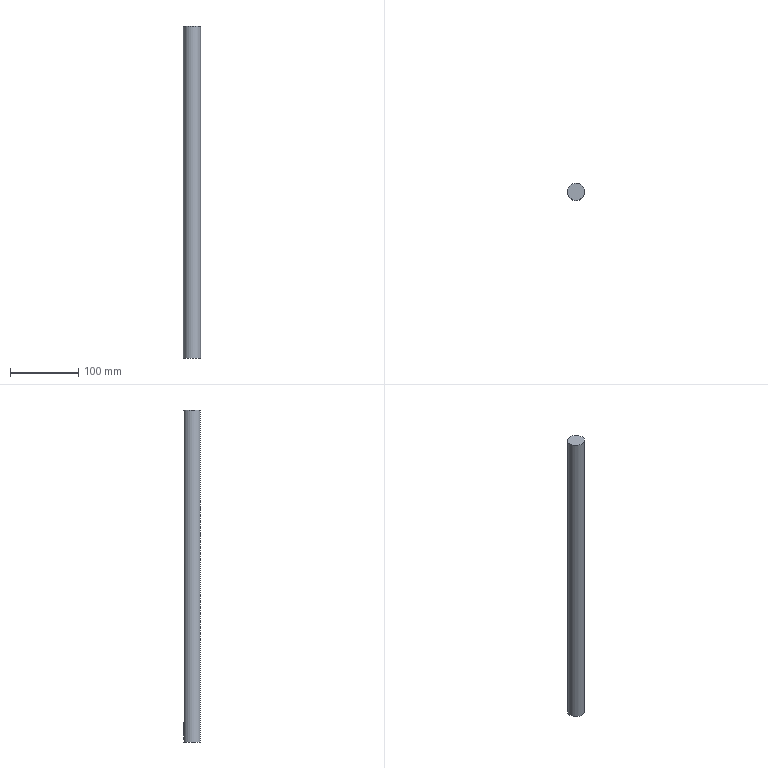Part | NX | 1 solid | 8 faces | box 25 x 25 x 487 mm | volume 238257 mm3 | plane 5 | cylinder 3 | commonest cylinder face diameters 8 x2 25 x1
STEP:
#1=CARTESIAN_POINT('',(-4.,11.843,-462.25));
#2=VERTEX_POINT('',#1);
#3=CARTESIAN_POINT('',(-4.,11.843,-479.75));
#4=VERTEX_POINT('',#3);
#5=CARTESIAN_POINT('',(-4.,11.843,0.));
#6=DIRECTION('',(0.,0.,-1.));
#7=VECTOR('',#6,1000.);
#8=LINE('',#5,#7);
#9=EDGE_CURVE('',#2,#4,#8,.T.);
#10=ORIENTED_EDGE('',*,*,#9,.T.);
#11=CARTESIAN_POINT('',(4.,11.843,-479.75));
#12=VERTEX_POINT('',#11);
#13=CARTESIAN_POINT('',(-4.,11.843,-479.75));
#14=CARTESIAN_POINT('',(-4.,11.843,-480.814));
#15=CARTESIAN_POINT('',(-3.133,12.18,-482.874));
#16=CARTESIAN_POINT('',(-0.006695,12.66,-484.187));
#17=CARTESIAN_POINT('',(3.135,12.181,-482.876));
#18=CARTESIAN_POINT('',(4.,11.843,-480.814));
#19=CARTESIAN_POINT('',(4.,11.843,-479.75));
#20=B_SPLINE_CURVE_WITH_KNOTS('',3,(#13,#14,#15,#16,#17,#18,#19),.UNSPECIFIED.,.F.,.F.,(4,1,1,1,4),(0.,0.003146,0.006292,0.009438,0.01258),.UNSPECIFIED.);
#21=EDGE_CURVE('',#4,#12,#20,.T.);
#22=ORIENTED_EDGE('',*,*,#21,.T.);
#23=CARTESIAN_POINT('',(4.,11.843,-462.25));
#24=VERTEX_POINT('',#23);
#25=CARTESIAN_POINT('',(4.,11.843,0.));
#26=DIRECTION('',(0.,0.,-1.));
#27=VECTOR('',#26,1000.);
#28=LINE('',#25,#27);
#29=EDGE_CURVE('',#12,#24,#28,.F.);
#30=ORIENTED_EDGE('',*,*,#29,.T.);
#31=CARTESIAN_POINT('',(4.,11.843,-462.25));
#32=CARTESIAN_POINT('',(4.,11.843,-461.186));
#33=CARTESIAN_POINT('',(3.133,12.18,-459.126));
#34=CARTESIAN_POINT('',(0.006695,12.66,-457.813));
#35=CARTESIAN_POINT('',(-3.135,12.181,-459.124));
#36=CARTESIAN_POINT('',(-4.,11.843,-461.186));
#37=CARTESIAN_POINT('',(-4.,11.843,-462.25));
#38=B_SPLINE_CURVE_WITH_KNOTS('',3,(#31,#32,#33,#34,#35,#36,#37),.UNSPECIFIED.,.F.,.F.,(4,1,1,1,4),(0.,0.003146,0.006292,0.009438,0.01258),.UNSPECIFIED.);
#39=EDGE_CURVE('',#24,#2,#38,.T.);
#40=ORIENTED_EDGE('',*,*,#39,.T.);
#41=EDGE_LOOP('',(#10,#22,#30,#40));
#42=FACE_BOUND('',#41,.T.);
#43=CARTESIAN_POINT('',(12.5,0.,0.));
#44=VERTEX_POINT('',#43);
#45=CARTESIAN_POINT('',(0.,0.,0.));
#46=DIRECTION('',(0.,0.,1.));
#47=DIRECTION('',(1.,0.,0.));
#48=AXIS2_PLACEMENT_3D('',#45,#46,#47);
#49=CIRCLE('',#48,12.5);
#50=EDGE_CURVE('',#44,#44,#49,.T.);
#51=ORIENTED_EDGE('',*,*,#50,.F.);
#52=EDGE_LOOP('',(#51));
#53=FACE_BOUND('',#52,.T.);
#54=CARTESIAN_POINT('',(12.5,0.,-487.));
#55=VERTEX_POINT('',#54);
#56=CARTESIAN_POINT('',(0.,0.,-487.));
#57=DIRECTION('',(0.,0.,1.));
#58=DIRECTION('',(1.,0.,0.));
#59=AXIS2_PLACEMENT_3D('',#56,#57,#58);
#60=CIRCLE('',#59,12.5);
#61=EDGE_CURVE('',#55,#55,#60,.T.);
#62=ORIENTED_EDGE('',*,*,#61,.T.);
#63=EDGE_LOOP('',(#62));
#64=FACE_BOUND('',#63,.T.);
#65=CARTESIAN_POINT('',(0.,0.,0.));
#66=DIRECTION('',(0.,0.,-1.));
#67=DIRECTION('',(-1.,0.,0.));
#68=AXIS2_PLACEMENT_3D('',#65,#66,#67);
#69=CYLINDRICAL_SURFACE('',#68,12.5);
#70=ADVANCED_FACE('',(#42,#53,#64),#69,.T.);
#71=ORIENTED_EDGE('',*,*,#50,.T.);
#72=EDGE_LOOP('',(#71));
#73=FACE_BOUND('',#72,.T.);
#74=CARTESIAN_POINT('',(0.,0.,0.));
#75=DIRECTION('',(0.,0.,1.));
#76=DIRECTION('',(1.,0.,0.));
#77=AXIS2_PLACEMENT_3D('',#74,#75,#76);
#78=PLANE('',#77);
#79=ADVANCED_FACE('',(#73),#78,.T.);
#80=ORIENTED_EDGE('',*,*,#61,.F.);
#81=EDGE_LOOP('',(#80));
#82=FACE_BOUND('',#81,.T.);
#83=CARTESIAN_POINT('',(0.,0.,-487.));
#84=DIRECTION('',(0.,0.,1.));
#85=DIRECTION('',(1.,0.,0.));
#86=AXIS2_PLACEMENT_3D('',#83,#84,#85);
#87=PLANE('',#86);
#88=ADVANCED_FACE('',(#82),#87,.F.);
#89=CARTESIAN_POINT('',(4.,8.1,-479.75));
#90=VERTEX_POINT('',#89);
#91=CARTESIAN_POINT('',(4.,12.5,-479.75));
#92=DIRECTION('',(0.,-1.,0.));
#93=VECTOR('',#92,1000.);
#94=LINE('',#91,#93);
#95=EDGE_CURVE('',#90,#12,#94,.F.);
#96=ORIENTED_EDGE('',*,*,#95,.F.);
#97=CARTESIAN_POINT('',(4.,8.1,-462.25));
#98=VERTEX_POINT('',#97);
#99=CARTESIAN_POINT('',(4.,8.1,-479.75));
#100=DIRECTION('',(0.,0.,1.));
#101=VECTOR('',#100,1000.);
#102=LINE('',#99,#101);
#103=EDGE_CURVE('',#98,#90,#102,.F.);
#104=ORIENTED_EDGE('',*,*,#103,.F.);
#105=CARTESIAN_POINT('',(4.,12.5,-462.25));
#106=DIRECTION('',(0.,-1.,0.));
#107=VECTOR('',#106,1000.);
#108=LINE('',#105,#107);
#109=EDGE_CURVE('',#98,#24,#108,.F.);
#110=ORIENTED_EDGE('',*,*,#109,.T.);
#111=ORIENTED_EDGE('',*,*,#29,.F.);
#112=EDGE_LOOP('',(#96,#104,#110,#111));
#113=FACE_BOUND('',#112,.T.);
#114=CARTESIAN_POINT('',(4.,12.5,-479.75));
#115=DIRECTION('',(1.,0.,0.));
#116=DIRECTION('',(0.,0.,-1.));
#117=AXIS2_PLACEMENT_3D('',#114,#115,#116);
#118=PLANE('',#117);
#119=ADVANCED_FACE('',(#113),#118,.F.);
#120=ORIENTED_EDGE('',*,*,#109,.F.);
#121=CARTESIAN_POINT('',(-4.,8.1,-462.25));
#122=VERTEX_POINT('',#121);
#123=CARTESIAN_POINT('',(0.,8.1,-462.25));
#124=DIRECTION('',(0.,-1.,0.));
#125=DIRECTION('',(0.,0.,1.));
#126=AXIS2_PLACEMENT_3D('',#123,#124,#125);
#127=CIRCLE('',#126,4.);
#128=EDGE_CURVE('',#122,#98,#127,.F.);
#129=ORIENTED_EDGE('',*,*,#128,.F.);
#130=CARTESIAN_POINT('',(-4.,12.5,-462.25));
#131=DIRECTION('',(0.,-1.,0.));
#132=VECTOR('',#131,1000.);
#133=LINE('',#130,#132);
#134=EDGE_CURVE('',#122,#2,#133,.F.);
#135=ORIENTED_EDGE('',*,*,#134,.T.);
#136=ORIENTED_EDGE('',*,*,#39,.F.);
#137=EDGE_LOOP('',(#120,#129,#135,#136));
#138=FACE_BOUND('',#137,.T.);
#139=CARTESIAN_POINT('',(0.,12.5,-462.25));
#140=DIRECTION('',(0.,-1.,0.));
#141=DIRECTION('',(0.,0.,-1.));
#142=AXIS2_PLACEMENT_3D('',#139,#140,#141);
#143=CYLINDRICAL_SURFACE('',#142,4.);
#144=ADVANCED_FACE('',(#138),#143,.F.);
#145=ORIENTED_EDGE('',*,*,#134,.F.);
#146=CARTESIAN_POINT('',(-4.,8.1,-479.75));
#147=VERTEX_POINT('',#146);
#148=CARTESIAN_POINT('',(-4.,8.1,-462.25));
#149=DIRECTION('',(0.,0.,-1.));
#150=VECTOR('',#149,1000.);
#151=LINE('',#148,#150);
#152=EDGE_CURVE('',#147,#122,#151,.F.);
#153=ORIENTED_EDGE('',*,*,#152,.F.);
#154=CARTESIAN_POINT('',(-4.,12.5,-479.75));
#155=DIRECTION('',(0.,-1.,0.));
#156=VECTOR('',#155,1000.);
#157=LINE('',#154,#156);
#158=EDGE_CURVE('',#147,#4,#157,.F.);
#159=ORIENTED_EDGE('',*,*,#158,.T.);
#160=ORIENTED_EDGE('',*,*,#9,.F.);
#161=EDGE_LOOP('',(#145,#153,#159,#160));
#162=FACE_BOUND('',#161,.T.);
#163=CARTESIAN_POINT('',(-4.,12.5,-462.25));
#164=DIRECTION('',(-1.,0.,0.));
#165=DIRECTION('',(0.,0.,1.));
#166=AXIS2_PLACEMENT_3D('',#163,#164,#165);
#167=PLANE('',#166);
#168=ADVANCED_FACE('',(#162),#167,.F.);
#169=ORIENTED_EDGE('',*,*,#158,.F.);
#170=CARTESIAN_POINT('',(0.,8.1,-479.75));
#171=DIRECTION('',(0.,-1.,0.));
#172=DIRECTION('',(0.,0.,1.));
#173=AXIS2_PLACEMENT_3D('',#170,#171,#172);
#174=CIRCLE('',#173,4.);
#175=EDGE_CURVE('',#90,#147,#174,.F.);
#176=ORIENTED_EDGE('',*,*,#175,.F.);
#177=ORIENTED_EDGE('',*,*,#95,.T.);
#178=ORIENTED_EDGE('',*,*,#21,.F.);
#179=EDGE_LOOP('',(#169,#176,#177,#178));
#180=FACE_BOUND('',#179,.T.);
#181=CARTESIAN_POINT('',(0.,12.5,-479.75));
#182=DIRECTION('',(0.,-1.,0.));
#183=DIRECTION('',(0.,0.,-1.));
#184=AXIS2_PLACEMENT_3D('',#181,#182,#183);
#185=CYLINDRICAL_SURFACE('',#184,4.);
#186=ADVANCED_FACE('',(#180),#185,.F.);
#187=ORIENTED_EDGE('',*,*,#103,.T.);
#188=ORIENTED_EDGE('',*,*,#175,.T.);
#189=ORIENTED_EDGE('',*,*,#152,.T.);
#190=ORIENTED_EDGE('',*,*,#128,.T.);
#191=EDGE_LOOP('',(#187,#188,#189,#190));
#192=FACE_BOUND('',#191,.T.);
#193=CARTESIAN_POINT('',(0.,8.1,-462.25));
#194=DIRECTION('',(0.,-1.,0.));
#195=DIRECTION('',(0.,0.,-1.));
#196=AXIS2_PLACEMENT_3D('',#193,#194,#195);
#197=PLANE('',#196);
#198=ADVANCED_FACE('',(#192),#197,.F.);
#199=CLOSED_SHELL('',(#70,#79,#88,#119,#144,#168,#186,#198));
#200=MANIFOLD_SOLID_BREP('',#199);
#201=(LENGTH_UNIT()NAMED_UNIT(*)SI_UNIT(.MILLI.,.METRE.));
#202=UNCERTAINTY_MEASURE_WITH_UNIT(LENGTH_MEASURE(0.0508),#201,'','');
#203=(NAMED_UNIT(*)PLANE_ANGLE_UNIT()SI_UNIT($,.RADIAN.));
#204=(NAMED_UNIT(*)SI_UNIT($,.STERADIAN.)SOLID_ANGLE_UNIT());
#205=(GEOMETRIC_REPRESENTATION_CONTEXT(3)GLOBAL_UNCERTAINTY_ASSIGNED_CONTEXT((#202))GLOBAL_UNIT_ASSIGNED_CONTEXT((#201,#203,#204))REPRESENTATION_CONTEXT('',''));
#206=ADVANCED_BREP_SHAPE_REPRESENTATION('',(#200),#205);